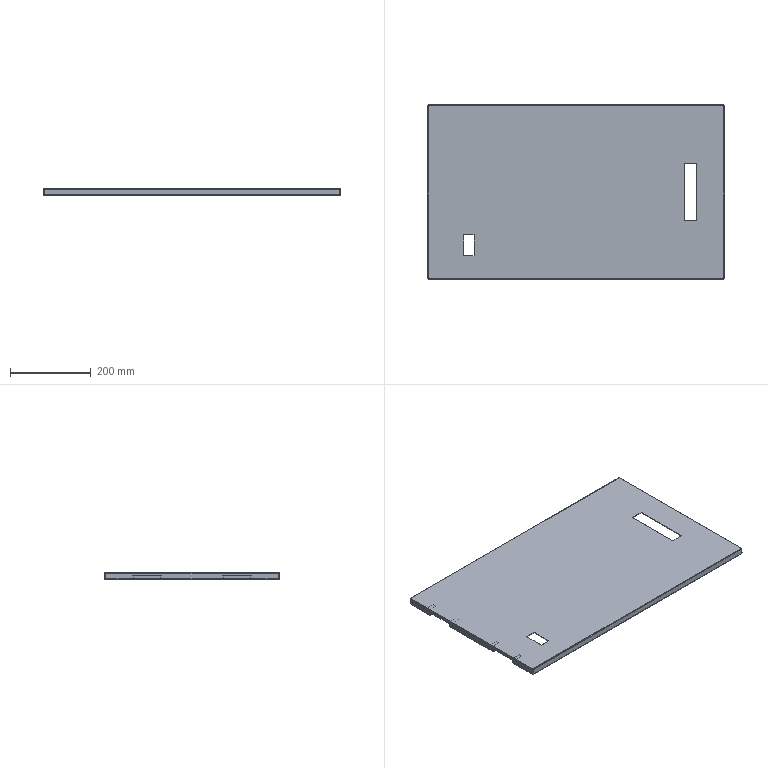Part | NX | features BREP 3 | 3 solids | 182 faces | box 736 x 432 x 16.5 mm | volume 550052 mm3 | plane 118 | cylinder 48 | spline 16 | commonest cylinder face diameters 0.02 x18 3.02 x18 3.2 x12